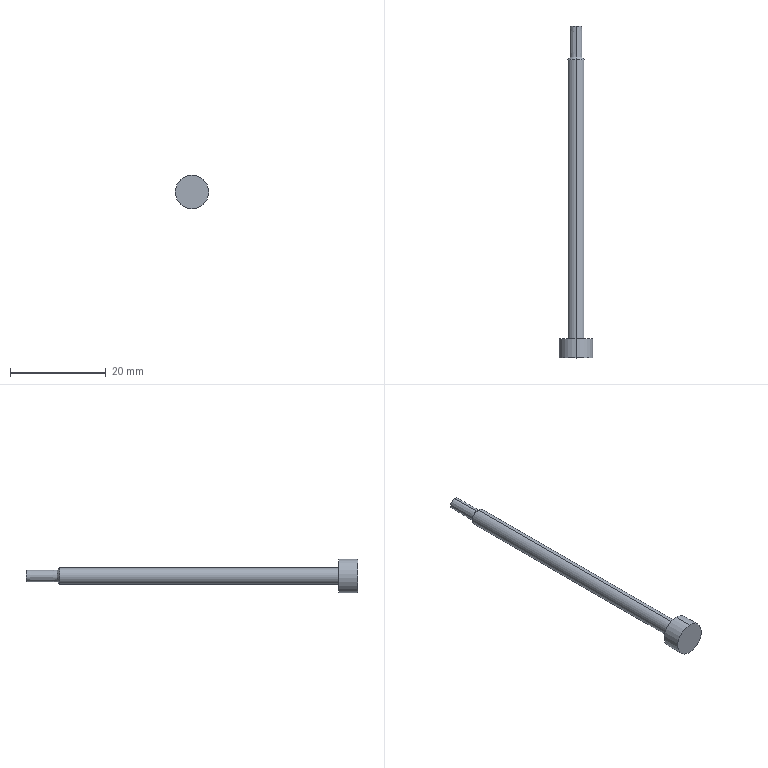Part | STEP file | 1 solid | 11 faces | box 7 x 69.447 x 7 mm | volume 750.263 mm3 | cylinder 4 | cone 4 | plane 3 | commonest cylinder face diameters 3.5 x2 7 x2
STEP:
#1=CARTESIAN_POINT('',(0.,0.,0.));
#2=DIRECTION('',(0.,0.,1.));
#3=DIRECTION('',(1.,0.,0.));
#4=AXIS2_PLACEMENT_3D('',#1,#2,#3);
#5=CARTESIAN_POINT('',(-30.652,-40.,49.73));
#6=VERTEX_POINT('',#5);
#7=CARTESIAN_POINT('',(-30.652,-40.,42.73));
#8=VERTEX_POINT('',#7);
#9=CARTESIAN_POINT('',(-30.652,-40.,46.23));
#10=DIRECTION('',(0.,1.,0.));
#11=DIRECTION('',(0.,0.,-1.));
#12=AXIS2_PLACEMENT_3D('',#9,#10,#11);
#13=CIRCLE('',#12,3.5);
#14=CARTESIAN_POINT('',(-30.652,-50.,46.23));
#15=DIRECTION('',(0.,1.,0.));
#16=DIRECTION('',(0.,0.,1.));
#17=AXIS2_PLACEMENT_3D('',#14,#15,#16);
#18=CYLINDRICAL_SURFACE('',#17,3.5);
#19=CARTESIAN_POINT('',(-3.142,10.));
#20=DIRECTION('',(1.,0.));
#21=VECTOR('',#20,1.);
#22=LINE('',#19,#21);
#23=(GEOMETRIC_REPRESENTATION_CONTEXT(2)PARAMETRIC_REPRESENTATION_CONTEXT()REPRESENTATION_CONTEXT('',''));
#24=DEFINITIONAL_REPRESENTATION('',(#22),#23);
#25=PCURVE('',#18,#24);
#26=CARTESIAN_POINT('',(-72.862,-40.,23.556));
#27=DIRECTION('',(0.,-1.,0.));
#28=DIRECTION('',(0.,0.,-1.));
#29=AXIS2_PLACEMENT_3D('',#26,#27,#28);
#30=PLANE('',#29);
#31=CARTESIAN_POINT('',(-19.174,42.21));
#32=CARTESIAN_POINT('',(-19.174,36.148));
#33=CARTESIAN_POINT('',(-24.424,39.179));
#34=CARTESIAN_POINT('',(-29.674,42.21));
#35=CARTESIAN_POINT('',(-24.424,45.241));
#36=CARTESIAN_POINT('',(-19.174,48.272));
#37=CARTESIAN_POINT('',(-19.174,42.21));
#38=(BOUNDED_CURVE()B_SPLINE_CURVE(2,(#31,#32,#33,#34,#35,#36,#37),.UNSPECIFIED.,.T.,.F.)B_SPLINE_CURVE_WITH_KNOTS((1,2,2,2,2,1),(-2.094,0.,2.094,4.189,6.283,8.378),.UNSPECIFIED.)CURVE()GEOMETRIC_REPRESENTATION_ITEM()RATIONAL_B_SPLINE_CURVE((1.,0.5,1.,0.5,1.,0.5,1.))REPRESENTATION_ITEM(''));
#39=(GEOMETRIC_REPRESENTATION_CONTEXT(2)PARAMETRIC_REPRESENTATION_CONTEXT()REPRESENTATION_CONTEXT('',''));
#40=DEFINITIONAL_REPRESENTATION('',(#38),#39);
#41=PCURVE('',#30,#40);
#42=SURFACE_CURVE('',#13,(#25,#41),.PCURVE_S1.);
#43=EDGE_CURVE('',#6,#8,#42,.T.);
#44=ORIENTED_EDGE('',*,*,#43,.T.);
#45=CARTESIAN_POINT('',(-30.652,-36.,42.73));
#46=VERTEX_POINT('',#45);
#47=CARTESIAN_POINT('',(-30.652,-50.,42.73));
#48=DIRECTION('',(0.,1.,0.));
#49=VECTOR('',#48,1.);
#50=LINE('',#47,#49);
#51=CARTESIAN_POINT('',(3.142,0.));
#52=DIRECTION('',(0.,1.));
#53=VECTOR('',#52,1.);
#54=LINE('',#51,#53);
#55=(GEOMETRIC_REPRESENTATION_CONTEXT(2)PARAMETRIC_REPRESENTATION_CONTEXT()REPRESENTATION_CONTEXT('',''));
#56=DEFINITIONAL_REPRESENTATION('',(#54),#55);
#57=PCURVE('',#18,#56);
#58=CARTESIAN_POINT('',(-30.652,-50.,46.23));
#59=DIRECTION('',(0.,1.,0.));
#60=DIRECTION('',(0.,0.,1.));
#61=AXIS2_PLACEMENT_3D('',#58,#59,#60);
#62=CYLINDRICAL_SURFACE('',#61,3.5);
#63=CARTESIAN_POINT('',(3.142,0.));
#64=DIRECTION('',(0.,1.));
#65=VECTOR('',#64,1.);
#66=LINE('',#63,#65);
#67=(GEOMETRIC_REPRESENTATION_CONTEXT(2)PARAMETRIC_REPRESENTATION_CONTEXT()REPRESENTATION_CONTEXT('',''));
#68=DEFINITIONAL_REPRESENTATION('',(#66),#67);
#69=PCURVE('',#62,#68);
#70=SURFACE_CURVE('',#50,(#57,#69),.PCURVE_S1.);
#71=EDGE_CURVE('',#8,#46,#70,.T.);
#72=ORIENTED_EDGE('',*,*,#71,.T.);
#73=CARTESIAN_POINT('',(-30.652,-36.,49.73));
#74=VERTEX_POINT('',#73);
#75=CARTESIAN_POINT('',(-30.652,-36.,46.23));
#76=DIRECTION('',(0.,-1.,0.));
#77=DIRECTION('',(0.,0.,-1.));
#78=AXIS2_PLACEMENT_3D('',#75,#76,#77);
#79=CIRCLE('',#78,3.5);
#80=CARTESIAN_POINT('',(3.142,14.));
#81=DIRECTION('',(-1.,0.));
#82=VECTOR('',#81,1.);
#83=LINE('',#80,#82);
#84=(GEOMETRIC_REPRESENTATION_CONTEXT(2)PARAMETRIC_REPRESENTATION_CONTEXT()REPRESENTATION_CONTEXT('',''));
#85=DEFINITIONAL_REPRESENTATION('',(#83),#84);
#86=PCURVE('',#18,#85);
#87=CARTESIAN_POINT('',(-30.652,-36.,46.23));
#88=DIRECTION('',(0.,1.,0.));
#89=DIRECTION('',(0.,0.,1.));
#90=AXIS2_PLACEMENT_3D('',#87,#88,#89);
#91=PLANE('',#90);
#92=CARTESIAN_POINT('',(-3.5,0.));
#93=CARTESIAN_POINT('',(-3.5,6.062));
#94=CARTESIAN_POINT('',(1.75,3.031));
#95=CARTESIAN_POINT('',(7.,0.));
#96=CARTESIAN_POINT('',(1.75,-3.031));
#97=CARTESIAN_POINT('',(-3.5,-6.062));
#98=CARTESIAN_POINT('',(-3.5,0.));
#99=(BOUNDED_CURVE()B_SPLINE_CURVE(2,(#92,#93,#94,#95,#96,#97,#98),.UNSPECIFIED.,.T.,.F.)B_SPLINE_CURVE_WITH_KNOTS((1,2,2,2,2,1),(-2.094,0.,2.094,4.189,6.283,8.378),.UNSPECIFIED.)CURVE()GEOMETRIC_REPRESENTATION_ITEM()RATIONAL_B_SPLINE_CURVE((1.,0.5,1.,0.5,1.,0.5,1.))REPRESENTATION_ITEM(''));
#100=(GEOMETRIC_REPRESENTATION_CONTEXT(2)PARAMETRIC_REPRESENTATION_CONTEXT()REPRESENTATION_CONTEXT('',''));
#101=DEFINITIONAL_REPRESENTATION('',(#99),#100);
#102=PCURVE('',#91,#101);
#103=SURFACE_CURVE('',#79,(#86,#102),.PCURVE_S1.);
#104=EDGE_CURVE('',#46,#74,#103,.T.);
#105=ORIENTED_EDGE('',*,*,#104,.T.);
#106=CARTESIAN_POINT('',(-30.652,-50.,49.73));
#107=DIRECTION('',(0.,1.,0.));
#108=VECTOR('',#107,1.);
#109=LINE('',#106,#108);
#110=CARTESIAN_POINT('',(0.,0.));
#111=DIRECTION('',(0.,1.));
#112=VECTOR('',#111,1.);
#113=LINE('',#110,#112);
#114=(GEOMETRIC_REPRESENTATION_CONTEXT(2)PARAMETRIC_REPRESENTATION_CONTEXT()REPRESENTATION_CONTEXT('',''));
#115=DEFINITIONAL_REPRESENTATION('',(#113),#114);
#116=PCURVE('',#18,#115);
#117=CARTESIAN_POINT('',(6.283,0.));
#118=DIRECTION('',(0.,1.));
#119=VECTOR('',#118,1.);
#120=LINE('',#117,#119);
#121=(GEOMETRIC_REPRESENTATION_CONTEXT(2)PARAMETRIC_REPRESENTATION_CONTEXT()REPRESENTATION_CONTEXT('',''));
#122=DEFINITIONAL_REPRESENTATION('',(#120),#121);
#123=PCURVE('',#62,#122);
#124=SURFACE_CURVE('',#109,(#116,#123),.PCURVE_S1.);
#125=EDGE_CURVE('',#6,#74,#124,.T.);
#126=ORIENTED_EDGE('',*,*,#125,.F.);
#127=EDGE_LOOP('',(#44,#72,#105,#126));
#128=FACE_BOUND('',#127,.T.);
#129=ADVANCED_FACE('',(#128),#18,.T.);
#130=CARTESIAN_POINT('',(-30.652,22.42,47.98));
#131=VERTEX_POINT('',#130);
#132=CARTESIAN_POINT('',(-30.652,22.42,44.48));
#133=VERTEX_POINT('',#132);
#134=CARTESIAN_POINT('',(-30.652,22.42,46.23));
#135=DIRECTION('',(0.,1.,0.));
#136=DIRECTION('',(0.,0.,-1.));
#137=AXIS2_PLACEMENT_3D('',#134,#135,#136);
#138=CIRCLE('',#137,1.75);
#139=CARTESIAN_POINT('',(-30.652,29.447,46.23));
#140=DIRECTION('',(0.,-1.,0.));
#141=DIRECTION('',(0.,0.,-1.));
#142=AXIS2_PLACEMENT_3D('',#139,#140,#141);
#143=CYLINDRICAL_SURFACE('',#142,1.75);
#144=CARTESIAN_POINT('',(6.283,7.026));
#145=DIRECTION('',(-1.,0.));
#146=VECTOR('',#145,1.);
#147=LINE('',#144,#146);
#148=(GEOMETRIC_REPRESENTATION_CONTEXT(2)PARAMETRIC_REPRESENTATION_CONTEXT()REPRESENTATION_CONTEXT('',''));
#149=DEFINITIONAL_REPRESENTATION('',(#147),#148);
#150=PCURVE('',#143,#149);
#151=CARTESIAN_POINT('',(-30.652,22.918,46.23));
#152=DIRECTION('',(0.,-1.,0.));
#153=DIRECTION('',(0.,0.,-1.));
#154=AXIS2_PLACEMENT_3D('',#151,#152,#153);
#155=CONICAL_SURFACE('',#154,1.252,0.7854);
#156=CARTESIAN_POINT('',(6.283,0.4982));
#157=DIRECTION('',(-1.,0.));
#158=VECTOR('',#157,1.);
#159=LINE('',#156,#158);
#160=(GEOMETRIC_REPRESENTATION_CONTEXT(2)PARAMETRIC_REPRESENTATION_CONTEXT()REPRESENTATION_CONTEXT('',''));
#161=DEFINITIONAL_REPRESENTATION('',(#159),#160);
#162=PCURVE('',#155,#161);
#163=SURFACE_CURVE('',#138,(#150,#162),.PCURVE_S1.);
#164=EDGE_CURVE('',#131,#133,#163,.T.);
#165=ORIENTED_EDGE('',*,*,#164,.F.);
#166=CARTESIAN_POINT('',(-30.652,-36.,47.98));
#167=VERTEX_POINT('',#166);
#168=CARTESIAN_POINT('',(-30.652,29.447,47.98));
#169=DIRECTION('',(0.,-1.,0.));
#170=VECTOR('',#169,1.);
#171=LINE('',#168,#170);
#172=CARTESIAN_POINT('',(3.142,0.));
#173=DIRECTION('',(0.,1.));
#174=VECTOR('',#173,1.);
#175=LINE('',#172,#174);
#176=(GEOMETRIC_REPRESENTATION_CONTEXT(2)PARAMETRIC_REPRESENTATION_CONTEXT()REPRESENTATION_CONTEXT('',''));
#177=DEFINITIONAL_REPRESENTATION('',(#175),#176);
#178=PCURVE('',#143,#177);
#179=CARTESIAN_POINT('',(-30.652,29.447,46.23));
#180=DIRECTION('',(0.,-1.,0.));
#181=DIRECTION('',(0.,0.,-1.));
#182=AXIS2_PLACEMENT_3D('',#179,#180,#181);
#183=CYLINDRICAL_SURFACE('',#182,1.75);
#184=CARTESIAN_POINT('',(3.142,0.));
#185=DIRECTION('',(0.,1.));
#186=VECTOR('',#185,1.);
#187=LINE('',#184,#186);
#188=(GEOMETRIC_REPRESENTATION_CONTEXT(2)PARAMETRIC_REPRESENTATION_CONTEXT()REPRESENTATION_CONTEXT('',''));
#189=DEFINITIONAL_REPRESENTATION('',(#187),#188);
#190=PCURVE('',#183,#189);
#191=SURFACE_CURVE('',#171,(#178,#190),.PCURVE_S1.);
#192=EDGE_CURVE('',#131,#167,#191,.T.);
#193=ORIENTED_EDGE('',*,*,#192,.T.);
#194=CARTESIAN_POINT('',(-30.652,-36.,44.48));
#195=VERTEX_POINT('',#194);
#196=CARTESIAN_POINT('',(-30.652,-36.,46.23));
#197=DIRECTION('',(0.,-1.,0.));
#198=DIRECTION('',(0.,0.,1.));
#199=AXIS2_PLACEMENT_3D('',#196,#197,#198);
#200=CIRCLE('',#199,1.75);
#201=CARTESIAN_POINT('',(-3.142,65.447));
#202=DIRECTION('',(1.,0.));
#203=VECTOR('',#202,1.);
#204=LINE('',#201,#203);
#205=(GEOMETRIC_REPRESENTATION_CONTEXT(2)PARAMETRIC_REPRESENTATION_CONTEXT()REPRESENTATION_CONTEXT('',''));
#206=DEFINITIONAL_REPRESENTATION('',(#204),#205);
#207=PCURVE('',#143,#206);
#208=CARTESIAN_POINT('',(1.75,0.));
#209=CARTESIAN_POINT('',(1.75,-3.031));
#210=CARTESIAN_POINT('',(-0.875,-1.516));
#211=CARTESIAN_POINT('',(-3.5,0.));
#212=CARTESIAN_POINT('',(-0.875,1.516));
#213=CARTESIAN_POINT('',(1.75,3.031));
#214=CARTESIAN_POINT('',(1.75,0.));
#215=(BOUNDED_CURVE()B_SPLINE_CURVE(2,(#208,#209,#210,#211,#212,#213,#214),.UNSPECIFIED.,.T.,.F.)B_SPLINE_CURVE_WITH_KNOTS((1,2,2,2,2,1),(-2.094,0.,2.094,4.189,6.283,8.378),.UNSPECIFIED.)CURVE()GEOMETRIC_REPRESENTATION_ITEM()RATIONAL_B_SPLINE_CURVE((1.,0.5,1.,0.5,1.,0.5,1.))REPRESENTATION_ITEM(''));
#216=(GEOMETRIC_REPRESENTATION_CONTEXT(2)PARAMETRIC_REPRESENTATION_CONTEXT()REPRESENTATION_CONTEXT('',''));
#217=DEFINITIONAL_REPRESENTATION('',(#215),#216);
#218=PCURVE('',#91,#217);
#219=SURFACE_CURVE('',#200,(#207,#218),.PCURVE_S1.);
#220=EDGE_CURVE('',#195,#167,#219,.T.);
#221=ORIENTED_EDGE('',*,*,#220,.F.);
#222=CARTESIAN_POINT('',(-30.652,29.447,44.48));
#223=DIRECTION('',(0.,-1.,0.));
#224=VECTOR('',#223,1.);
#225=LINE('',#222,#224);
#226=CARTESIAN_POINT('',(0.,0.));
#227=DIRECTION('',(0.,1.));
#228=VECTOR('',#227,1.);
#229=LINE('',#226,#228);
#230=(GEOMETRIC_REPRESENTATION_CONTEXT(2)PARAMETRIC_REPRESENTATION_CONTEXT()REPRESENTATION_CONTEXT('',''));
#231=DEFINITIONAL_REPRESENTATION('',(#229),#230);
#232=PCURVE('',#143,#231);
#233=CARTESIAN_POINT('',(6.283,0.));
#234=DIRECTION('',(0.,1.));
#235=VECTOR('',#234,1.);
#236=LINE('',#233,#235);
#237=(GEOMETRIC_REPRESENTATION_CONTEXT(2)PARAMETRIC_REPRESENTATION_CONTEXT()REPRESENTATION_CONTEXT('',''));
#238=DEFINITIONAL_REPRESENTATION('',(#236),#237);
#239=PCURVE('',#183,#238);
#240=SURFACE_CURVE('',#225,(#232,#239),.PCURVE_S1.);
#241=EDGE_CURVE('',#133,#195,#240,.T.);
#242=ORIENTED_EDGE('',*,*,#241,.F.);
#243=EDGE_LOOP('',(#165,#193,#221,#242));
#244=FACE_BOUND('',#243,.T.);
#245=ADVANCED_FACE('',(#244),#143,.T.);
#246=CARTESIAN_POINT('',(-30.652,29.447,45.035));
#247=VERTEX_POINT('',#246);
#248=CARTESIAN_POINT('',(-30.652,29.447,47.425));
#249=VERTEX_POINT('',#248);
#250=CARTESIAN_POINT('',(-30.652,29.447,46.23));
#251=DIRECTION('',(0.,-1.,0.));
#252=DIRECTION('',(0.,0.,-1.));
#253=AXIS2_PLACEMENT_3D('',#250,#251,#252);
#254=CIRCLE('',#253,1.195);
#255=CARTESIAN_POINT('',(-30.652,22.412,46.23));
#256=DIRECTION('',(0.,-1.,0.));
#257=DIRECTION('',(0.,0.,-1.));
#258=AXIS2_PLACEMENT_3D('',#255,#256,#257);
#259=CONICAL_SURFACE('',#258,1.256,0.008727);
#260=CARTESIAN_POINT('',(0.,-7.035));
#261=DIRECTION('',(1.,0.));
#262=VECTOR('',#261,1.);
#263=LINE('',#260,#262);
#264=(GEOMETRIC_REPRESENTATION_CONTEXT(2)PARAMETRIC_REPRESENTATION_CONTEXT()REPRESENTATION_CONTEXT('',''));
#265=DEFINITIONAL_REPRESENTATION('',(#263),#264);
#266=PCURVE('',#259,#265);
#267=CARTESIAN_POINT('',(-30.652,29.447,46.23));
#268=DIRECTION('',(0.,1.,0.));
#269=DIRECTION('',(0.,0.,1.));
#270=AXIS2_PLACEMENT_3D('',#267,#268,#269);
#271=PLANE('',#270);
#272=CARTESIAN_POINT('',(-1.195,0.));
#273=CARTESIAN_POINT('',(-1.195,2.07));
#274=CARTESIAN_POINT('',(0.5974,1.035));
#275=CARTESIAN_POINT('',(2.39,0.));
#276=CARTESIAN_POINT('',(0.5974,-1.035));
#277=CARTESIAN_POINT('',(-1.195,-2.07));
#278=CARTESIAN_POINT('',(-1.195,0.));
#279=(BOUNDED_CURVE()B_SPLINE_CURVE(2,(#272,#273,#274,#275,#276,#277,#278),.UNSPECIFIED.,.T.,.F.)B_SPLINE_CURVE_WITH_KNOTS((1,2,2,2,2,1),(-2.094,0.,2.094,4.189,6.283,8.378),.UNSPECIFIED.)CURVE()GEOMETRIC_REPRESENTATION_ITEM()RATIONAL_B_SPLINE_CURVE((1.,0.5,1.,0.5,1.,0.5,1.))REPRESENTATION_ITEM(''));
#280=(GEOMETRIC_REPRESENTATION_CONTEXT(2)PARAMETRIC_REPRESENTATION_CONTEXT()REPRESENTATION_CONTEXT('',''));
#281=DEFINITIONAL_REPRESENTATION('',(#279),#280);
#282=PCURVE('',#271,#281);
#283=SURFACE_CURVE('',#254,(#266,#282),.PCURVE_S1.);
#284=EDGE_CURVE('',#247,#249,#283,.T.);
#285=ORIENTED_EDGE('',*,*,#284,.T.);
#286=CARTESIAN_POINT('',(-30.652,22.918,47.482));
#287=VERTEX_POINT('',#286);
#288=CARTESIAN_POINT('',(-30.652,22.412,47.486));
#289=DIRECTION('',(0.,-1.,0.008727));
#290=VECTOR('',#289,1.);
#291=LINE('',#288,#290);
#292=CARTESIAN_POINT('',(3.142,0.));
#293=DIRECTION('',(0.,1.));
#294=VECTOR('',#293,1.);
#295=LINE('',#292,#294);
#296=(GEOMETRIC_REPRESENTATION_CONTEXT(2)PARAMETRIC_REPRESENTATION_CONTEXT()REPRESENTATION_CONTEXT('',''));
#297=DEFINITIONAL_REPRESENTATION('',(#295),#296);
#298=PCURVE('',#259,#297);
#299=CARTESIAN_POINT('',(-30.652,22.412,46.23));
#300=DIRECTION('',(0.,-1.,0.));
#301=DIRECTION('',(0.,0.,-1.));
#302=AXIS2_PLACEMENT_3D('',#299,#300,#301);
#303=CONICAL_SURFACE('',#302,1.256,0.008727);
#304=CARTESIAN_POINT('',(3.142,0.));
#305=DIRECTION('',(0.,1.));
#306=VECTOR('',#305,1.);
#307=LINE('',#304,#306);
#308=(GEOMETRIC_REPRESENTATION_CONTEXT(2)PARAMETRIC_REPRESENTATION_CONTEXT()REPRESENTATION_CONTEXT('',''));
#309=DEFINITIONAL_REPRESENTATION('',(#307),#308);
#310=PCURVE('',#303,#309);
#311=SURFACE_CURVE('',#291,(#298,#310),.PCURVE_S1.);
#312=EDGE_CURVE('',#249,#287,#311,.T.);
#313=ORIENTED_EDGE('',*,*,#312,.T.);
#314=CARTESIAN_POINT('',(-30.652,22.918,44.978));
#315=VERTEX_POINT('',#314);
#316=CARTESIAN_POINT('',(-30.652,22.918,46.23));
#317=DIRECTION('',(0.,-1.,0.));
#318=DIRECTION('',(0.,0.,-1.));
#319=AXIS2_PLACEMENT_3D('',#316,#317,#318);
#320=CIRCLE('',#319,1.252);
#321=CARTESIAN_POINT('',(0.,-0.5069));
#322=DIRECTION('',(1.,0.));
#323=VECTOR('',#322,1.);
#324=LINE('',#321,#323);
#325=(GEOMETRIC_REPRESENTATION_CONTEXT(2)PARAMETRIC_REPRESENTATION_CONTEXT()REPRESENTATION_CONTEXT('',''));
#326=DEFINITIONAL_REPRESENTATION('',(#324),#325);
#327=PCURVE('',#259,#326);
#328=CARTESIAN_POINT('',(0.,0.));
#329=DIRECTION('',(1.,0.));
#330=VECTOR('',#329,1.);
#331=LINE('',#328,#330);
#332=(GEOMETRIC_REPRESENTATION_CONTEXT(2)PARAMETRIC_REPRESENTATION_CONTEXT()REPRESENTATION_CONTEXT('',''));
#333=DEFINITIONAL_REPRESENTATION('',(#331),#332);
#334=PCURVE('',#155,#333);
#335=SURFACE_CURVE('',#320,(#327,#334),.PCURVE_S1.);
#336=EDGE_CURVE('',#315,#287,#335,.T.);
#337=ORIENTED_EDGE('',*,*,#336,.F.);
#338=CARTESIAN_POINT('',(-30.652,22.412,44.974));
#339=DIRECTION('',(0.,-1.,-0.008727));
#340=VECTOR('',#339,1.);
#341=LINE('',#338,#340);
#342=CARTESIAN_POINT('',(0.,0.));
#343=DIRECTION('',(0.,1.));
#344=VECTOR('',#343,1.);
#345=LINE('',#342,#344);
#346=(GEOMETRIC_REPRESENTATION_CONTEXT(2)PARAMETRIC_REPRESENTATION_CONTEXT()REPRESENTATION_CONTEXT('',''));
#347=DEFINITIONAL_REPRESENTATION('',(#345),#346);
#348=PCURVE('',#259,#347);
#349=CARTESIAN_POINT('',(6.283,0.));
#350=DIRECTION('',(0.,1.));
#351=VECTOR('',#350,1.);
#352=LINE('',#349,#351);
#353=(GEOMETRIC_REPRESENTATION_CONTEXT(2)PARAMETRIC_REPRESENTATION_CONTEXT()REPRESENTATION_CONTEXT('',''));
#354=DEFINITIONAL_REPRESENTATION('',(#352),#353);
#355=PCURVE('',#303,#354);
#356=SURFACE_CURVE('',#341,(#348,#355),.PCURVE_S1.);
#357=EDGE_CURVE('',#247,#315,#356,.T.);
#358=ORIENTED_EDGE('',*,*,#357,.F.);
#359=EDGE_LOOP('',(#285,#313,#337,#358));
#360=FACE_BOUND('',#359,.T.);
#361=ADVANCED_FACE('',(#360),#259,.T.);
#362=ORIENTED_EDGE('',*,*,#336,.T.);
#363=CARTESIAN_POINT('',(-30.652,22.918,47.482));
#364=DIRECTION('',(0.,-0.7071,0.7071));
#365=VECTOR('',#364,1.);
#366=LINE('',#363,#365);
#367=CARTESIAN_POINT('',(3.142,0.));
#368=DIRECTION('',(0.,1.));
#369=VECTOR('',#368,1.);
#370=LINE('',#367,#369);
#371=(GEOMETRIC_REPRESENTATION_CONTEXT(2)PARAMETRIC_REPRESENTATION_CONTEXT()REPRESENTATION_CONTEXT('',''));
#372=DEFINITIONAL_REPRESENTATION('',(#370),#371);
#373=PCURVE('',#155,#372);
#374=CARTESIAN_POINT('',(-30.652,22.918,46.23));
#375=DIRECTION('',(0.,-1.,0.));
#376=DIRECTION('',(0.,0.,-1.));
#377=AXIS2_PLACEMENT_3D('',#374,#375,#376);
#378=CONICAL_SURFACE('',#377,1.252,0.7854);
#379=CARTESIAN_POINT('',(3.142,0.));
#380=DIRECTION('',(0.,1.));
#381=VECTOR('',#380,1.);
#382=LINE('',#379,#381);
#383=(GEOMETRIC_REPRESENTATION_CONTEXT(2)PARAMETRIC_REPRESENTATION_CONTEXT()REPRESENTATION_CONTEXT('',''));
#384=DEFINITIONAL_REPRESENTATION('',(#382),#383);
#385=PCURVE('',#378,#384);
#386=SURFACE_CURVE('',#366,(#373,#385),.PCURVE_S1.);
#387=EDGE_CURVE('',#287,#131,#386,.T.);
#388=ORIENTED_EDGE('',*,*,#387,.T.);
#389=ORIENTED_EDGE('',*,*,#164,.T.);
#390=CARTESIAN_POINT('',(-30.652,22.918,44.978));
#391=DIRECTION('',(0.,-0.7071,-0.7071));
#392=VECTOR('',#391,1.);
#393=LINE('',#390,#392);
#394=CARTESIAN_POINT('',(0.,0.));
#395=DIRECTION('',(0.,1.));
#396=VECTOR('',#395,1.);
#397=LINE('',#394,#396);
#398=(GEOMETRIC_REPRESENTATION_CONTEXT(2)PARAMETRIC_REPRESENTATION_CONTEXT()REPRESENTATION_CONTEXT('',''));
#399=DEFINITIONAL_REPRESENTATION('',(#397),#398);
#400=PCURVE('',#155,#399);
#401=CARTESIAN_POINT('',(6.283,0.));
#402=DIRECTION('',(0.,1.));
#403=VECTOR('',#402,1.);
#404=LINE('',#401,#403);
#405=(GEOMETRIC_REPRESENTATION_CONTEXT(2)PARAMETRIC_REPRESENTATION_CONTEXT()REPRESENTATION_CONTEXT('',''));
#406=DEFINITIONAL_REPRESENTATION('',(#404),#405);
#407=PCURVE('',#378,#406);
#408=SURFACE_CURVE('',#393,(#400,#407),.PCURVE_S1.);
#409=EDGE_CURVE('',#315,#133,#408,.T.);
#410=ORIENTED_EDGE('',*,*,#409,.F.);
#411=EDGE_LOOP('',(#362,#388,#389,#410));
#412=FACE_BOUND('',#411,.T.);
#413=ADVANCED_FACE('',(#412),#155,.T.);
#414=ORIENTED_EDGE('',*,*,#387,.F.);
#415=CARTESIAN_POINT('',(-30.652,22.918,46.23));
#416=DIRECTION('',(0.,-1.,0.));
#417=DIRECTION('',(0.,0.,-1.));
#418=AXIS2_PLACEMENT_3D('',#415,#416,#417);
#419=CIRCLE('',#418,1.252);
#420=CARTESIAN_POINT('',(0.,0.));
#421=DIRECTION('',(1.,0.));
#422=VECTOR('',#421,1.);
#423=LINE('',#420,#422);
#424=(GEOMETRIC_REPRESENTATION_CONTEXT(2)PARAMETRIC_REPRESENTATION_CONTEXT()REPRESENTATION_CONTEXT('',''));
#425=DEFINITIONAL_REPRESENTATION('',(#423),#424);
#426=PCURVE('',#378,#425);
#427=CARTESIAN_POINT('',(0.,-0.5069));
#428=DIRECTION('',(1.,0.));
#429=VECTOR('',#428,1.);
#430=LINE('',#427,#429);
#431=(GEOMETRIC_REPRESENTATION_CONTEXT(2)PARAMETRIC_REPRESENTATION_CONTEXT()REPRESENTATION_CONTEXT('',''));
#432=DEFINITIONAL_REPRESENTATION('',(#430),#431);
#433=PCURVE('',#303,#432);
#434=SURFACE_CURVE('',#419,(#426,#433),.PCURVE_S1.);
#435=EDGE_CURVE('',#287,#315,#434,.T.);
#436=ORIENTED_EDGE('',*,*,#435,.T.);
#437=ORIENTED_EDGE('',*,*,#409,.T.);
#438=CARTESIAN_POINT('',(-30.652,22.42,46.23));
#439=DIRECTION('',(0.,1.,0.));
#440=DIRECTION('',(0.,0.,-1.));
#441=AXIS2_PLACEMENT_3D('',#438,#439,#440);
#442=CIRCLE('',#441,1.75);
#443=CARTESIAN_POINT('',(6.283,0.4982));
#444=DIRECTION('',(-1.,0.));
#445=VECTOR('',#444,1.);
#446=LINE('',#443,#445);
#447=(GEOMETRIC_REPRESENTATION_CONTEXT(2)PARAMETRIC_REPRESENTATION_CONTEXT()REPRESENTATION_CONTEXT('',''));
#448=DEFINITIONAL_REPRESENTATION('',(#446),#447);
#449=PCURVE('',#378,#448);
#450=CARTESIAN_POINT('',(6.283,7.026));
#451=DIRECTION('',(-1.,0.));
#452=VECTOR('',#451,1.);
#453=LINE('',#450,#452);
#454=(GEOMETRIC_REPRESENTATION_CONTEXT(2)PARAMETRIC_REPRESENTATION_CONTEXT()REPRESENTATION_CONTEXT('',''));
#455=DEFINITIONAL_REPRESENTATION('',(#453),#454);
#456=PCURVE('',#183,#455);
#457=SURFACE_CURVE('',#442,(#449,#456),.PCURVE_S1.);
#458=EDGE_CURVE('',#133,#131,#457,.T.);
#459=ORIENTED_EDGE('',*,*,#458,.T.);
#460=EDGE_LOOP('',(#414,#436,#437,#459));
#461=FACE_BOUND('',#460,.T.);
#462=ADVANCED_FACE('',(#461),#378,.T.);
#463=ORIENTED_EDGE('',*,*,#312,.F.);
#464=CARTESIAN_POINT('',(-30.652,29.447,46.23));
#465=DIRECTION('',(0.,-1.,0.));
#466=DIRECTION('',(0.,0.,-1.));
#467=AXIS2_PLACEMENT_3D('',#464,#465,#466);
#468=CIRCLE('',#467,1.195);
#469=CARTESIAN_POINT('',(0.,-7.035));
#470=DIRECTION('',(1.,0.));
#471=VECTOR('',#470,1.);
#472=LINE('',#469,#471);
#473=(GEOMETRIC_REPRESENTATION_CONTEXT(2)PARAMETRIC_REPRESENTATION_CONTEXT()REPRESENTATION_CONTEXT('',''));
#474=DEFINITIONAL_REPRESENTATION('',(#472),#473);
#475=PCURVE('',#303,#474);
#476=CARTESIAN_POINT('',(-1.195,0.));
#477=CARTESIAN_POINT('',(-1.195,2.07));
#478=CARTESIAN_POINT('',(0.5974,1.035));
#479=CARTESIAN_POINT('',(2.39,0.));
#480=CARTESIAN_POINT('',(0.5974,-1.035));
#481=CARTESIAN_POINT('',(-1.195,-2.07));
#482=CARTESIAN_POINT('',(-1.195,0.));
#483=(BOUNDED_CURVE()B_SPLINE_CURVE(2,(#476,#477,#478,#479,#480,#481,#482),.UNSPECIFIED.,.T.,.F.)B_SPLINE_CURVE_WITH_KNOTS((1,2,2,2,2,1),(-2.094,0.,2.094,4.189,6.283,8.378),.UNSPECIFIED.)CURVE()GEOMETRIC_REPRESENTATION_ITEM()RATIONAL_B_SPLINE_CURVE((1.,0.5,1.,0.5,1.,0.5,1.))REPRESENTATION_ITEM(''));
#484=(GEOMETRIC_REPRESENTATION_CONTEXT(2)PARAMETRIC_REPRESENTATION_CONTEXT()REPRESENTATION_CONTEXT('',''));
#485=DEFINITIONAL_REPRESENTATION('',(#483),#484);
#486=PCURVE('',#271,#485);
#487=SURFACE_CURVE('',#468,(#475,#486),.PCURVE_S1.);
#488=EDGE_CURVE('',#249,#247,#487,.T.);
#489=ORIENTED_EDGE('',*,*,#488,.T.);
#490=ORIENTED_EDGE('',*,*,#357,.T.);
#491=ORIENTED_EDGE('',*,*,#435,.F.);
#492=EDGE_LOOP('',(#463,#489,#490,#491));
#493=FACE_BOUND('',#492,.T.);
#494=ADVANCED_FACE('',(#493),#303,.T.);
#495=ORIENTED_EDGE('',*,*,#192,.F.);
#496=ORIENTED_EDGE('',*,*,#458,.F.);
#497=ORIENTED_EDGE('',*,*,#241,.T.);
#498=CARTESIAN_POINT('',(-30.652,-36.,46.23));
#499=DIRECTION('',(0.,-1.,0.));
#500=DIRECTION('',(0.,0.,1.));
#501=AXIS2_PLACEMENT_3D('',#498,#499,#500);
#502=CIRCLE('',#501,1.75);
#503=CARTESIAN_POINT('',(3.142,65.447));
#504=DIRECTION('',(1.,0.));
#505=VECTOR('',#504,1.);
#506=LINE('',#503,#505);
#507=(GEOMETRIC_REPRESENTATION_CONTEXT(2)PARAMETRIC_REPRESENTATION_CONTEXT()REPRESENTATION_CONTEXT('',''));
#508=DEFINITIONAL_REPRESENTATION('',(#506),#507);
#509=PCURVE('',#183,#508);
#510=CARTESIAN_POINT('',(1.75,0.));
#511=CARTESIAN_POINT('',(1.75,-3.031));
#512=CARTESIAN_POINT('',(-0.875,-1.516));
#513=CARTESIAN_POINT('',(-3.5,0.));
#514=CARTESIAN_POINT('',(-0.875,1.516));
#515=CARTESIAN_POINT('',(1.75,3.031));
#516=CARTESIAN_POINT('',(1.75,0.));
#517=(BOUNDED_CURVE()B_SPLINE_CURVE(2,(#510,#511,#512,#513,#514,#515,#516),.UNSPECIFIED.,.T.,.F.)B_SPLINE_CURVE_WITH_KNOTS((1,2,2,2,2,1),(-2.094,0.,2.094,4.189,6.283,8.378),.UNSPECIFIED.)CURVE()GEOMETRIC_REPRESENTATION_ITEM()RATIONAL_B_SPLINE_CURVE((1.,0.5,1.,0.5,1.,0.5,1.))REPRESENTATION_ITEM(''));
#518=(GEOMETRIC_REPRESENTATION_CONTEXT(2)PARAMETRIC_REPRESENTATION_CONTEXT()REPRESENTATION_CONTEXT('',''));
#519=DEFINITIONAL_REPRESENTATION('',(#517),#518);
#520=PCURVE('',#91,#519);
#521=SURFACE_CURVE('',#502,(#509,#520),.PCURVE_S1.);
#522=EDGE_CURVE('',#167,#195,#521,.T.);
#523=ORIENTED_EDGE('',*,*,#522,.F.);
#524=EDGE_LOOP('',(#495,#496,#497,#523));
#525=FACE_BOUND('',#524,.T.);
#526=ADVANCED_FACE('',(#525),#183,.T.);
#527=ORIENTED_EDGE('',*,*,#284,.F.);
#528=ORIENTED_EDGE('',*,*,#488,.F.);
#529=EDGE_LOOP('',(#527,#528));
#530=FACE_BOUND('',#529,.T.);
#531=ADVANCED_FACE('',(#530),#271,.T.);
#532=ORIENTED_EDGE('',*,*,#220,.T.);
#533=ORIENTED_EDGE('',*,*,#522,.T.);
#534=EDGE_LOOP('',(#532,#533));
#535=FACE_BOUND('',#534,.T.);
#536=CARTESIAN_POINT('',(-30.652,-36.,46.23));
#537=DIRECTION('',(0.,-1.,0.));
#538=DIRECTION('',(0.,0.,-1.));
#539=AXIS2_PLACEMENT_3D('',#536,#537,#538);
#540=CIRCLE('',#539,3.5);
#541=CARTESIAN_POINT('',(-3.5,0.));
#542=CARTESIAN_POINT('',(-3.5,6.062));
#543=CARTESIAN_POINT('',(1.75,3.031));
#544=CARTESIAN_POINT('',(7.,0.));
#545=CARTESIAN_POINT('',(1.75,-3.031));
#546=CARTESIAN_POINT('',(-3.5,-6.062));
#547=CARTESIAN_POINT('',(-3.5,0.));
#548=(BOUNDED_CURVE()B_SPLINE_CURVE(2,(#541,#542,#543,#544,#545,#546,#547),.UNSPECIFIED.,.T.,.F.)B_SPLINE_CURVE_WITH_KNOTS((1,2,2,2,2,1),(-2.094,0.,2.094,4.189,6.283,8.378),.UNSPECIFIED.)CURVE()GEOMETRIC_REPRESENTATION_ITEM()RATIONAL_B_SPLINE_CURVE((1.,0.5,1.,0.5,1.,0.5,1.))REPRESENTATION_ITEM(''));
#549=(GEOMETRIC_REPRESENTATION_CONTEXT(2)PARAMETRIC_REPRESENTATION_CONTEXT()REPRESENTATION_CONTEXT('',''));
#550=DEFINITIONAL_REPRESENTATION('',(#548),#549);
#551=PCURVE('',#91,#550);
#552=CARTESIAN_POINT('',(9.425,14.));
#553=DIRECTION('',(-1.,0.));
#554=VECTOR('',#553,1.);
#555=LINE('',#552,#554);
#556=(GEOMETRIC_REPRESENTATION_CONTEXT(2)PARAMETRIC_REPRESENTATION_CONTEXT()REPRESENTATION_CONTEXT('',''));
#557=DEFINITIONAL_REPRESENTATION('',(#555),#556);
#558=PCURVE('',#62,#557);
#559=SURFACE_CURVE('',#540,(#551,#558),.PCURVE_S1.);
#560=EDGE_CURVE('',#74,#46,#559,.T.);
#561=ORIENTED_EDGE('',*,*,#560,.F.);
#562=ORIENTED_EDGE('',*,*,#104,.F.);
#563=EDGE_LOOP('',(#561,#562));
#564=FACE_BOUND('',#563,.T.);
#565=ADVANCED_FACE('',(#535,#564),#91,.T.);
#566=ORIENTED_EDGE('',*,*,#71,.F.);
#567=CARTESIAN_POINT('',(-30.652,-40.,46.23));
#568=DIRECTION('',(0.,1.,0.));
#569=DIRECTION('',(0.,0.,-1.));
#570=AXIS2_PLACEMENT_3D('',#567,#568,#569);
#571=CIRCLE('',#570,3.5);
#572=CARTESIAN_POINT('',(3.142,10.));
#573=DIRECTION('',(1.,0.));
#574=VECTOR('',#573,1.);
#575=LINE('',#572,#574);
#576=(GEOMETRIC_REPRESENTATION_CONTEXT(2)PARAMETRIC_REPRESENTATION_CONTEXT()REPRESENTATION_CONTEXT('',''));
#577=DEFINITIONAL_REPRESENTATION('',(#575),#576);
#578=PCURVE('',#62,#577);
#579=CARTESIAN_POINT('',(-19.174,42.21));
#580=CARTESIAN_POINT('',(-19.174,36.148));
#581=CARTESIAN_POINT('',(-24.424,39.179));
#582=CARTESIAN_POINT('',(-29.674,42.21));
#583=CARTESIAN_POINT('',(-24.424,45.241));
#584=CARTESIAN_POINT('',(-19.174,48.272));
#585=CARTESIAN_POINT('',(-19.174,42.21));
#586=(BOUNDED_CURVE()B_SPLINE_CURVE(2,(#579,#580,#581,#582,#583,#584,#585),.UNSPECIFIED.,.T.,.F.)B_SPLINE_CURVE_WITH_KNOTS((1,2,2,2,2,1),(-2.094,0.,2.094,4.189,6.283,8.378),.UNSPECIFIED.)CURVE()GEOMETRIC_REPRESENTATION_ITEM()RATIONAL_B_SPLINE_CURVE((1.,0.5,1.,0.5,1.,0.5,1.))REPRESENTATION_ITEM(''));
#587=(GEOMETRIC_REPRESENTATION_CONTEXT(2)PARAMETRIC_REPRESENTATION_CONTEXT()REPRESENTATION_CONTEXT('',''));
#588=DEFINITIONAL_REPRESENTATION('',(#586),#587);
#589=PCURVE('',#30,#588);
#590=SURFACE_CURVE('',#571,(#578,#589),.PCURVE_S1.);
#591=EDGE_CURVE('',#8,#6,#590,.T.);
#592=ORIENTED_EDGE('',*,*,#591,.T.);
#593=ORIENTED_EDGE('',*,*,#125,.T.);
#594=ORIENTED_EDGE('',*,*,#560,.T.);
#595=EDGE_LOOP('',(#566,#592,#593,#594));
#596=FACE_BOUND('',#595,.T.);
#597=ADVANCED_FACE('',(#596),#62,.T.);
#598=ORIENTED_EDGE('',*,*,#43,.F.);
#599=ORIENTED_EDGE('',*,*,#591,.F.);
#600=EDGE_LOOP('',(#598,#599));
#601=FACE_BOUND('',#600,.T.);
#602=ADVANCED_FACE('',(#601),#30,.T.);
#603=CLOSED_SHELL('',(#129,#245,#361,#413,#462,#494,#526,#531,#565,#597,#602));
#604=MANIFOLD_SOLID_BREP('',#603);
#605=(LENGTH_UNIT()NAMED_UNIT(*)SI_UNIT(.MILLI.,.METRE.));
#606=UNCERTAINTY_MEASURE_WITH_UNIT(LENGTH_MEASURE(0.0000001),#605,'','');
#607=(NAMED_UNIT(*)PLANE_ANGLE_UNIT()SI_UNIT($,.RADIAN.));
#608=(NAMED_UNIT(*)SI_UNIT($,.STERADIAN.)SOLID_ANGLE_UNIT());
#609=(GEOMETRIC_REPRESENTATION_CONTEXT(3)GLOBAL_UNCERTAINTY_ASSIGNED_CONTEXT((#606))GLOBAL_UNIT_ASSIGNED_CONTEXT((#605,#607,#608))REPRESENTATION_CONTEXT('',''));
#610=ADVANCED_BREP_SHAPE_REPRESENTATION('',(#4,#604),#609);